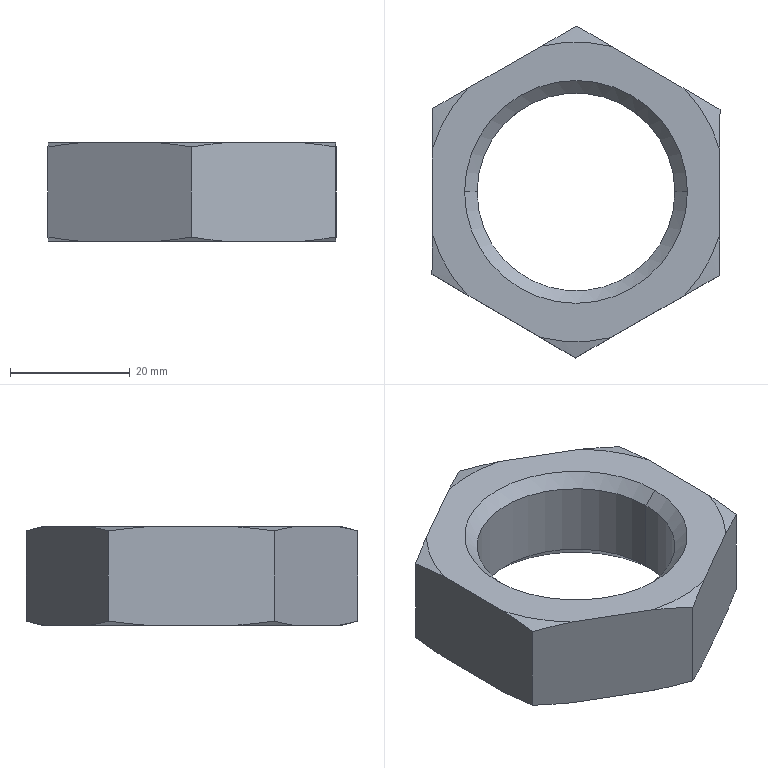Part | STEP file | GB/T 6173-M32×2_(M33) | 1 solid | 26 faces | box 48.06 x 55.37 x 16.5 mm | volume 18235 mm3 | cone 16 | plane 8 | cylinder 2 | commonest cylinder face diameters 33 x2
STEP:
#1=CARTESIAN_POINT('',(-16.5,0.,14.414));
#2=VERTEX_POINT('',#1);
#3=CARTESIAN_POINT('',(16.5,0.,14.414));
#4=VERTEX_POINT('',#3);
#5=CARTESIAN_POINT('',(0.,0.,14.414));
#6=DIRECTION('',(0.,0.,1.));
#7=DIRECTION('',(-1.,0.,0.));
#8=AXIS2_PLACEMENT_3D('',#5,#6,#7);
#9=CIRCLE('',#8,16.5);
#10=EDGE_CURVE('',#2,#4,#9,.T.);
#11=ORIENTED_EDGE('',*,*,#10,.F.);
#12=CARTESIAN_POINT('',(-18.586,0.,16.5));
#13=VERTEX_POINT('',#12);
#14=CARTESIAN_POINT('',(-16.5,0.,14.414));
#15=DIRECTION('',(-0.7071,0.,0.7071));
#16=VECTOR('',#15,1000.);
#17=LINE('',#14,#16);
#18=EDGE_CURVE('',#2,#13,#17,.T.);
#19=ORIENTED_EDGE('',*,*,#18,.T.);
#20=CARTESIAN_POINT('',(18.586,0.,16.5));
#21=VERTEX_POINT('',#20);
#22=CARTESIAN_POINT('',(0.,0.,16.5));
#23=DIRECTION('',(0.,0.,-1.));
#24=DIRECTION('',(-1.,0.,0.));
#25=AXIS2_PLACEMENT_3D('',#22,#23,#24);
#26=CIRCLE('',#25,18.586);
#27=EDGE_CURVE('',#21,#13,#26,.T.);
#28=ORIENTED_EDGE('',*,*,#27,.F.);
#29=CARTESIAN_POINT('',(16.5,0.,14.414));
#30=DIRECTION('',(0.7071,0.,0.7071));
#31=VECTOR('',#30,1000.);
#32=LINE('',#29,#31);
#33=EDGE_CURVE('',#4,#21,#32,.T.);
#34=ORIENTED_EDGE('',*,*,#33,.F.);
#35=EDGE_LOOP('',(#11,#19,#28,#34));
#36=FACE_OUTER_BOUND('',#35,.T.);
#37=CARTESIAN_POINT('',(0.,0.,14.414));
#38=DIRECTION('',(0.,0.,1.));
#39=DIRECTION('',(1.,0.,0.));
#40=AXIS2_PLACEMENT_3D('',#37,#38,#39);
#41=CONICAL_SURFACE('',#40,16.5,0.7854);
#42=ADVANCED_FACE('',(#36),#41,.F.);
#43=CARTESIAN_POINT('',(16.5,0.,2.086));
#44=VERTEX_POINT('',#43);
#45=CARTESIAN_POINT('',(-16.5,0.,2.086));
#46=VERTEX_POINT('',#45);
#47=CARTESIAN_POINT('',(0.,0.,2.086));
#48=DIRECTION('',(0.,0.,-1.));
#49=DIRECTION('',(-1.,0.,0.));
#50=AXIS2_PLACEMENT_3D('',#47,#48,#49);
#51=CIRCLE('',#50,16.5);
#52=EDGE_CURVE('',#44,#46,#51,.T.);
#53=ORIENTED_EDGE('',*,*,#52,.F.);
#54=CARTESIAN_POINT('',(18.586,0.,0.));
#55=VERTEX_POINT('',#54);
#56=CARTESIAN_POINT('',(18.586,0.,0.));
#57=DIRECTION('',(0.7071,0.,-0.7071));
#58=VECTOR('',#57,1000.);
#59=LINE('',#56,#58);
#60=EDGE_CURVE('',#44,#55,#59,.T.);
#61=ORIENTED_EDGE('',*,*,#60,.T.);
#62=CARTESIAN_POINT('',(-18.586,0.,0.));
#63=VERTEX_POINT('',#62);
#64=CARTESIAN_POINT('',(0.,0.,0.));
#65=DIRECTION('',(0.,0.,1.));
#66=DIRECTION('',(-1.,0.,0.));
#67=AXIS2_PLACEMENT_3D('',#64,#65,#66);
#68=CIRCLE('',#67,18.586);
#69=EDGE_CURVE('',#63,#55,#68,.T.);
#70=ORIENTED_EDGE('',*,*,#69,.F.);
#71=CARTESIAN_POINT('',(-18.586,0.,0.));
#72=DIRECTION('',(-0.7071,0.,-0.7071));
#73=VECTOR('',#72,1000.);
#74=LINE('',#71,#73);
#75=EDGE_CURVE('',#46,#63,#74,.T.);
#76=ORIENTED_EDGE('',*,*,#75,.F.);
#77=EDGE_LOOP('',(#53,#61,#70,#76));
#78=FACE_OUTER_BOUND('',#77,.T.);
#79=CARTESIAN_POINT('',(0.,0.,0.));
#80=DIRECTION('',(0.,0.,-1.));
#81=DIRECTION('',(-1.,0.,0.));
#82=AXIS2_PLACEMENT_3D('',#79,#80,#81);
#83=CONICAL_SURFACE('',#82,18.586,0.7854);
#84=ADVANCED_FACE('',(#78),#83,.F.);
#85=ORIENTED_EDGE('',*,*,#10,.T.);
#86=CARTESIAN_POINT('',(16.5,0.,16.5));
#87=DIRECTION('',(0.,0.,-1.));
#88=VECTOR('',#87,1000.);
#89=LINE('',#86,#88);
#90=EDGE_CURVE('',#4,#44,#89,.T.);
#91=ORIENTED_EDGE('',*,*,#90,.T.);
#92=ORIENTED_EDGE('',*,*,#52,.T.);
#93=CARTESIAN_POINT('',(-16.5,0.,16.5));
#94=DIRECTION('',(0.,0.,-1.));
#95=VECTOR('',#94,1000.);
#96=LINE('',#93,#95);
#97=EDGE_CURVE('',#2,#46,#96,.T.);
#98=ORIENTED_EDGE('',*,*,#97,.F.);
#99=EDGE_LOOP('',(#85,#91,#92,#98));
#100=FACE_OUTER_BOUND('',#99,.T.);
#101=CARTESIAN_POINT('',(0.,0.,16.5));
#102=DIRECTION('',(0.,0.,-1.));
#103=DIRECTION('',(-1.,0.,0.));
#104=AXIS2_PLACEMENT_3D('',#101,#102,#103);
#105=CYLINDRICAL_SURFACE('',#104,16.5);
#106=ADVANCED_FACE('',(#100),#105,.F.);
#107=CARTESIAN_POINT('',(24.03,13.748,15.781));
#108=VERTEX_POINT('',#107);
#109=CARTESIAN_POINT('',(18.189,17.151,16.5));
#110=VERTEX_POINT('',#109);
#111=CARTESIAN_POINT('',(24.03,13.748,15.781));
#112=CARTESIAN_POINT('',(22.089,14.879,16.082));
#113=CARTESIAN_POINT('',(20.142,16.013,16.328));
#114=CARTESIAN_POINT('',(18.189,17.151,16.5));
#115=B_SPLINE_CURVE_WITH_KNOTS('',3,(#111,#112,#113,#114),.UNSPECIFIED.,.F.,.F.,(4,4),(0.02271,0.02951),.UNSPECIFIED.);
#116=EDGE_CURVE('',#108,#110,#115,.T.);
#117=ORIENTED_EDGE('',*,*,#116,.F.);
#118=CARTESIAN_POINT('',(24.03,13.748,0.7194));
#119=VERTEX_POINT('',#118);
#120=CARTESIAN_POINT('',(24.03,13.748,16.5));
#121=DIRECTION('',(0.,0.,-1.));
#122=VECTOR('',#121,1000.);
#123=LINE('',#120,#122);
#124=EDGE_CURVE('',#108,#119,#123,.T.);
#125=ORIENTED_EDGE('',*,*,#124,.T.);
#126=CARTESIAN_POINT('',(18.189,17.151,0.));
#127=VERTEX_POINT('',#126);
#128=CARTESIAN_POINT('',(18.189,17.151,0.));
#129=CARTESIAN_POINT('',(19.165,16.582,0.08577));
#130=CARTESIAN_POINT('',(20.143,16.013,0.1906));
#131=CARTESIAN_POINT('',(22.09,14.879,0.4323));
#132=CARTESIAN_POINT('',(23.061,14.313,0.5692));
#133=CARTESIAN_POINT('',(24.03,13.748,0.7194));
#134=B_SPLINE_CURVE_WITH_KNOTS('',3,(#128,#129,#130,#131,#132,#133),.UNSPECIFIED.,.F.,.F.,(4,2,4),(0.04359,0.04693,0.05027),.UNSPECIFIED.);
#135=EDGE_CURVE('',#127,#119,#134,.T.);
#136=ORIENTED_EDGE('',*,*,#135,.F.);
#137=CARTESIAN_POINT('',(5.95,24.282,0.));
#138=VERTEX_POINT('',#137);
#139=CARTESIAN_POINT('',(24.03,13.748,0.));
#140=DIRECTION('',(-0.8641,0.5034,0.));
#141=VECTOR('',#140,1000.);
#142=LINE('',#139,#141);
#143=EDGE_CURVE('',#127,#138,#142,.T.);
#144=ORIENTED_EDGE('',*,*,#143,.T.);
#145=CARTESIAN_POINT('',(0.1089,27.685,0.7194));
#146=VERTEX_POINT('',#145);
#147=CARTESIAN_POINT('',(0.1089,27.685,0.7194));
#148=CARTESIAN_POINT('',(2.05,26.554,0.4184));
#149=CARTESIAN_POINT('',(3.997,25.42,0.1716));
#150=CARTESIAN_POINT('',(5.95,24.282,0.));
#151=B_SPLINE_CURVE_WITH_KNOTS('',3,(#147,#148,#149,#150),.UNSPECIFIED.,.F.,.F.,(4,4),(0.02271,0.02951),.UNSPECIFIED.);
#152=EDGE_CURVE('',#146,#138,#151,.T.);
#153=ORIENTED_EDGE('',*,*,#152,.F.);
#154=CARTESIAN_POINT('',(0.1089,27.685,15.781));
#155=VERTEX_POINT('',#154);
#156=CARTESIAN_POINT('',(0.1089,27.685,16.5));
#157=DIRECTION('',(0.,0.,-1.));
#158=VECTOR('',#157,1000.);
#159=LINE('',#156,#158);
#160=EDGE_CURVE('',#155,#146,#159,.T.);
#161=ORIENTED_EDGE('',*,*,#160,.F.);
#162=CARTESIAN_POINT('',(5.95,24.282,16.5));
#163=VERTEX_POINT('',#162);
#164=CARTESIAN_POINT('',(5.95,24.282,16.5));
#165=CARTESIAN_POINT('',(4.974,24.85,16.414));
#166=CARTESIAN_POINT('',(3.996,25.42,16.309));
#167=CARTESIAN_POINT('',(2.049,26.554,16.068));
#168=CARTESIAN_POINT('',(1.078,27.12,15.931));
#169=CARTESIAN_POINT('',(0.1089,27.685,15.781));
#170=B_SPLINE_CURVE_WITH_KNOTS('',3,(#164,#165,#166,#167,#168,#169),.UNSPECIFIED.,.F.,.F.,(4,2,4),(0.04359,0.04693,0.05027),.UNSPECIFIED.);
#171=EDGE_CURVE('',#163,#155,#170,.T.);
#172=ORIENTED_EDGE('',*,*,#171,.F.);
#173=CARTESIAN_POINT('',(24.03,13.748,16.5));
#174=DIRECTION('',(-0.8641,0.5034,0.));
#175=VECTOR('',#174,1000.);
#176=LINE('',#173,#175);
#177=EDGE_CURVE('',#110,#163,#176,.T.);
#178=ORIENTED_EDGE('',*,*,#177,.F.);
#179=EDGE_LOOP('',(#117,#125,#136,#144,#153,#161,#172,#178));
#180=FACE_OUTER_BOUND('',#179,.T.);
#181=CARTESIAN_POINT('',(24.03,13.748,16.5));
#182=DIRECTION('',(-0.5034,-0.8641,0.));
#183=DIRECTION('',(0.8641,-0.5034,0.));
#184=AXIS2_PLACEMENT_3D('',#181,#182,#183);
#185=PLANE('',#184);
#186=ADVANCED_FACE('',(#180),#185,.F.);
#187=CARTESIAN_POINT('',(-5.759,24.328,16.5));
#188=VERTEX_POINT('',#187);
#189=CARTESIAN_POINT('',(0.1089,27.685,15.781));
#190=CARTESIAN_POINT('',(-1.841,26.569,16.082));
#191=CARTESIAN_POINT('',(-3.797,25.45,16.328));
#192=CARTESIAN_POINT('',(-5.759,24.328,16.5));
#193=B_SPLINE_CURVE_WITH_KNOTS('',3,(#189,#190,#191,#192),.UNSPECIFIED.,.F.,.F.,(4,4),(0.0226,0.0294),.UNSPECIFIED.);
#194=EDGE_CURVE('',#155,#188,#193,.T.);
#195=ORIENTED_EDGE('',*,*,#194,.F.);
#196=ORIENTED_EDGE('',*,*,#160,.T.);
#197=CARTESIAN_POINT('',(-5.759,24.328,0.));
#198=VERTEX_POINT('',#197);
#199=CARTESIAN_POINT('',(-5.759,24.328,0.));
#200=CARTESIAN_POINT('',(-4.778,24.889,0.08577));
#201=CARTESIAN_POINT('',(-3.796,25.451,0.1906));
#202=CARTESIAN_POINT('',(-1.84,26.57,0.4323));
#203=CARTESIAN_POINT('',(-0.8647,27.128,0.5692));
#204=CARTESIAN_POINT('',(0.1089,27.685,0.7194));
#205=B_SPLINE_CURVE_WITH_KNOTS('',3,(#199,#200,#201,#202,#203,#204),.UNSPECIFIED.,.F.,.F.,(4,2,4),(0.04348,0.04682,0.05017),.UNSPECIFIED.);
#206=EDGE_CURVE('',#198,#146,#205,.T.);
#207=ORIENTED_EDGE('',*,*,#206,.F.);
#208=CARTESIAN_POINT('',(-18.053,17.294,0.));
#209=VERTEX_POINT('',#208);
#210=CARTESIAN_POINT('',(0.1089,27.685,0.));
#211=DIRECTION('',(-0.868,-0.4966,0.));
#212=VECTOR('',#211,1000.);
#213=LINE('',#210,#212);
#214=EDGE_CURVE('',#198,#209,#213,.T.);
#215=ORIENTED_EDGE('',*,*,#214,.T.);
#216=CARTESIAN_POINT('',(-23.921,13.937,0.7194));
#217=VERTEX_POINT('',#216);
#218=CARTESIAN_POINT('',(-23.921,13.937,0.7194));
#219=CARTESIAN_POINT('',(-21.971,15.052,0.4184));
#220=CARTESIAN_POINT('',(-20.016,16.171,0.1716));
#221=CARTESIAN_POINT('',(-18.053,17.294,0.));
#222=B_SPLINE_CURVE_WITH_KNOTS('',3,(#218,#219,#220,#221),.UNSPECIFIED.,.F.,.F.,(4,4),(0.0226,0.0294),.UNSPECIFIED.);
#223=EDGE_CURVE('',#217,#209,#222,.T.);
#224=ORIENTED_EDGE('',*,*,#223,.F.);
#225=CARTESIAN_POINT('',(-23.921,13.937,15.781));
#226=VERTEX_POINT('',#225);
#227=CARTESIAN_POINT('',(-23.921,13.937,16.5));
#228=DIRECTION('',(0.,0.,-1.));
#229=VECTOR('',#228,1000.);
#230=LINE('',#227,#229);
#231=EDGE_CURVE('',#226,#217,#230,.T.);
#232=ORIENTED_EDGE('',*,*,#231,.F.);
#233=CARTESIAN_POINT('',(-18.053,17.294,16.5));
#234=VERTEX_POINT('',#233);
#235=CARTESIAN_POINT('',(-18.053,17.294,16.5));
#236=CARTESIAN_POINT('',(-19.034,16.733,16.414));
#237=CARTESIAN_POINT('',(-20.016,16.171,16.309));
#238=CARTESIAN_POINT('',(-21.972,15.052,16.068));
#239=CARTESIAN_POINT('',(-22.948,14.494,15.931));
#240=CARTESIAN_POINT('',(-23.921,13.937,15.781));
#241=B_SPLINE_CURVE_WITH_KNOTS('',3,(#235,#236,#237,#238,#239,#240),.UNSPECIFIED.,.F.,.F.,(4,2,4),(0.04348,0.04682,0.05017),.UNSPECIFIED.);
#242=EDGE_CURVE('',#234,#226,#241,.T.);
#243=ORIENTED_EDGE('',*,*,#242,.F.);
#244=CARTESIAN_POINT('',(0.1089,27.685,16.5));
#245=DIRECTION('',(-0.868,-0.4966,0.));
#246=VECTOR('',#245,1000.);
#247=LINE('',#244,#246);
#248=EDGE_CURVE('',#188,#234,#247,.T.);
#249=ORIENTED_EDGE('',*,*,#248,.F.);
#250=EDGE_LOOP('',(#195,#196,#207,#215,#224,#232,#243,#249));
#251=FACE_OUTER_BOUND('',#250,.T.);
#252=CARTESIAN_POINT('',(0.1089,27.685,16.5));
#253=DIRECTION('',(0.4966,-0.868,0.));
#254=DIRECTION('',(0.868,0.4966,0.));
#255=AXIS2_PLACEMENT_3D('',#252,#253,#254);
#256=PLANE('',#255);
#257=ADVANCED_FACE('',(#251),#256,.F.);
#258=CARTESIAN_POINT('',(-23.948,7.176,16.5));
#259=VERTEX_POINT('',#258);
#260=CARTESIAN_POINT('',(-23.921,13.937,15.781));
#261=CARTESIAN_POINT('',(-23.93,11.689,16.082));
#262=CARTESIAN_POINT('',(-23.939,9.437,16.328));
#263=CARTESIAN_POINT('',(-23.948,7.176,16.5));
#264=B_SPLINE_CURVE_WITH_KNOTS('',3,(#260,#261,#262,#263),.UNSPECIFIED.,.F.,.F.,(4,4),(0.01959,0.02639),.UNSPECIFIED.);
#265=EDGE_CURVE('',#226,#259,#264,.T.);
#266=ORIENTED_EDGE('',*,*,#265,.F.);
#267=ORIENTED_EDGE('',*,*,#231,.T.);
#268=CARTESIAN_POINT('',(-23.948,7.176,0.));
#269=VERTEX_POINT('',#268);
#270=CARTESIAN_POINT('',(-23.948,7.176,0.));
#271=CARTESIAN_POINT('',(-23.943,8.305,0.08567));
#272=CARTESIAN_POINT('',(-23.939,9.436,0.1905));
#273=CARTESIAN_POINT('',(-23.93,11.69,0.4322));
#274=CARTESIAN_POINT('',(-23.926,12.815,0.5691));
#275=CARTESIAN_POINT('',(-23.921,13.937,0.7194));
#276=B_SPLINE_CURVE_WITH_KNOTS('',3,(#270,#271,#272,#273,#274,#275),.UNSPECIFIED.,.F.,.F.,(4,2,4),(0.04049,0.04383,0.04718),.UNSPECIFIED.);
#277=EDGE_CURVE('',#269,#217,#276,.T.);
#278=ORIENTED_EDGE('',*,*,#277,.F.);
#279=CARTESIAN_POINT('',(-24.004,-6.988,0.));
#280=VERTEX_POINT('',#279);
#281=CARTESIAN_POINT('',(-23.921,13.937,0.));
#282=DIRECTION('',(-0.003934,-1.,0.));
#283=VECTOR('',#282,1000.);
#284=LINE('',#281,#283);
#285=EDGE_CURVE('',#269,#280,#284,.T.);
#286=ORIENTED_EDGE('',*,*,#285,.T.);
#287=CARTESIAN_POINT('',(-24.03,-13.748,0.7194));
#288=VERTEX_POINT('',#287);
#289=CARTESIAN_POINT('',(-24.03,-13.748,0.7194));
#290=CARTESIAN_POINT('',(-24.021,-11.501,0.4184));
#291=CARTESIAN_POINT('',(-24.012,-9.248,0.1716));
#292=CARTESIAN_POINT('',(-24.004,-6.988,0.));
#293=B_SPLINE_CURVE_WITH_KNOTS('',3,(#289,#290,#291,#292),.UNSPECIFIED.,.F.,.F.,(4,4),(0.01959,0.02639),.UNSPECIFIED.);
#294=EDGE_CURVE('',#288,#280,#293,.T.);
#295=ORIENTED_EDGE('',*,*,#294,.F.);
#296=CARTESIAN_POINT('',(-24.03,-13.748,15.781));
#297=VERTEX_POINT('',#296);
#298=CARTESIAN_POINT('',(-24.03,-13.748,16.5));
#299=DIRECTION('',(0.,0.,-1.));
#300=VECTOR('',#299,1000.);
#301=LINE('',#298,#300);
#302=EDGE_CURVE('',#297,#288,#301,.T.);
#303=ORIENTED_EDGE('',*,*,#302,.F.);
#304=CARTESIAN_POINT('',(-24.004,-6.988,16.5));
#305=VERTEX_POINT('',#304);
#306=CARTESIAN_POINT('',(-24.004,-6.988,16.5));
#307=CARTESIAN_POINT('',(-24.008,-8.116,16.414));
#308=CARTESIAN_POINT('',(-24.012,-9.248,16.31));
#309=CARTESIAN_POINT('',(-24.021,-11.502,16.068));
#310=CARTESIAN_POINT('',(-24.026,-12.626,15.931));
#311=CARTESIAN_POINT('',(-24.03,-13.748,15.781));
#312=B_SPLINE_CURVE_WITH_KNOTS('',3,(#306,#307,#308,#309,#310,#311),.UNSPECIFIED.,.F.,.F.,(4,2,4),(0.04049,0.04383,0.04718),.UNSPECIFIED.);
#313=EDGE_CURVE('',#305,#297,#312,.T.);
#314=ORIENTED_EDGE('',*,*,#313,.F.);
#315=CARTESIAN_POINT('',(-23.921,13.937,16.5));
#316=DIRECTION('',(-0.003934,-1.,0.));
#317=VECTOR('',#316,1000.);
#318=LINE('',#315,#317);
#319=EDGE_CURVE('',#259,#305,#318,.T.);
#320=ORIENTED_EDGE('',*,*,#319,.F.);
#321=EDGE_LOOP('',(#266,#267,#278,#286,#295,#303,#314,#320));
#322=FACE_OUTER_BOUND('',#321,.T.);
#323=CARTESIAN_POINT('',(-23.921,13.937,16.5));
#324=DIRECTION('',(1.,-0.003934,0.));
#325=DIRECTION('',(0.003934,1.,0.));
#326=AXIS2_PLACEMENT_3D('',#323,#324,#325);
#327=PLANE('',#326);
#328=ADVANCED_FACE('',(#322),#327,.F.);
#329=CARTESIAN_POINT('',(-18.189,-17.151,16.5));
#330=VERTEX_POINT('',#329);
#331=CARTESIAN_POINT('',(-24.03,-13.748,15.781));
#332=CARTESIAN_POINT('',(-22.089,-14.879,16.082));
#333=CARTESIAN_POINT('',(-20.142,-16.013,16.328));
#334=CARTESIAN_POINT('',(-18.189,-17.151,16.5));
#335=B_SPLINE_CURVE_WITH_KNOTS('',3,(#331,#332,#333,#334),.UNSPECIFIED.,.F.,.F.,(4,4),(0.02271,0.02951),.UNSPECIFIED.);
#336=EDGE_CURVE('',#297,#330,#335,.T.);
#337=ORIENTED_EDGE('',*,*,#336,.F.);
#338=ORIENTED_EDGE('',*,*,#302,.T.);
#339=CARTESIAN_POINT('',(-18.189,-17.151,0.));
#340=VERTEX_POINT('',#339);
#341=CARTESIAN_POINT('',(-18.189,-17.151,0.));
#342=CARTESIAN_POINT('',(-19.165,-16.582,0.08577));
#343=CARTESIAN_POINT('',(-20.143,-16.013,0.1906));
#344=CARTESIAN_POINT('',(-22.09,-14.879,0.4323));
#345=CARTESIAN_POINT('',(-23.061,-14.313,0.5692));
#346=CARTESIAN_POINT('',(-24.03,-13.748,0.7194));
#347=B_SPLINE_CURVE_WITH_KNOTS('',3,(#341,#342,#343,#344,#345,#346),.UNSPECIFIED.,.F.,.F.,(4,2,4),(0.04359,0.04693,0.05027),.UNSPECIFIED.);
#348=EDGE_CURVE('',#340,#288,#347,.T.);
#349=ORIENTED_EDGE('',*,*,#348,.F.);
#350=CARTESIAN_POINT('',(-5.95,-24.282,0.));
#351=VERTEX_POINT('',#350);
#352=CARTESIAN_POINT('',(-24.03,-13.748,0.));
#353=DIRECTION('',(0.8641,-0.5034,0.));
#354=VECTOR('',#353,1000.);
#355=LINE('',#352,#354);
#356=EDGE_CURVE('',#340,#351,#355,.T.);
#357=ORIENTED_EDGE('',*,*,#356,.T.);
#358=CARTESIAN_POINT('',(-0.1089,-27.685,0.7194));
#359=VERTEX_POINT('',#358);
#360=CARTESIAN_POINT('',(-0.1089,-27.685,0.7194));
#361=CARTESIAN_POINT('',(-2.05,-26.554,0.4184));
#362=CARTESIAN_POINT('',(-3.997,-25.42,0.1716));
#363=CARTESIAN_POINT('',(-5.95,-24.282,0.));
#364=B_SPLINE_CURVE_WITH_KNOTS('',3,(#360,#361,#362,#363),.UNSPECIFIED.,.F.,.F.,(4,4),(0.02271,0.02951),.UNSPECIFIED.);
#365=EDGE_CURVE('',#359,#351,#364,.T.);
#366=ORIENTED_EDGE('',*,*,#365,.F.);
#367=CARTESIAN_POINT('',(-0.1089,-27.685,15.781));
#368=VERTEX_POINT('',#367);
#369=CARTESIAN_POINT('',(-0.1089,-27.685,16.5));
#370=DIRECTION('',(0.,0.,-1.));
#371=VECTOR('',#370,1000.);
#372=LINE('',#369,#371);
#373=EDGE_CURVE('',#368,#359,#372,.T.);
#374=ORIENTED_EDGE('',*,*,#373,.F.);
#375=CARTESIAN_POINT('',(-5.95,-24.282,16.5));
#376=VERTEX_POINT('',#375);
#377=CARTESIAN_POINT('',(-5.95,-24.282,16.5));
#378=CARTESIAN_POINT('',(-4.974,-24.85,16.414));
#379=CARTESIAN_POINT('',(-3.996,-25.42,16.309));
#380=CARTESIAN_POINT('',(-2.049,-26.554,16.068));
#381=CARTESIAN_POINT('',(-1.078,-27.12,15.931));
#382=CARTESIAN_POINT('',(-0.1089,-27.685,15.781));
#383=B_SPLINE_CURVE_WITH_KNOTS('',3,(#377,#378,#379,#380,#381,#382),.UNSPECIFIED.,.F.,.F.,(4,2,4),(0.04359,0.04693,0.05027),.UNSPECIFIED.);
#384=EDGE_CURVE('',#376,#368,#383,.T.);
#385=ORIENTED_EDGE('',*,*,#384,.F.);
#386=CARTESIAN_POINT('',(-24.03,-13.748,16.5));
#387=DIRECTION('',(0.8641,-0.5034,0.));
#388=VECTOR('',#387,1000.);
#389=LINE('',#386,#388);
#390=EDGE_CURVE('',#330,#376,#389,.T.);
#391=ORIENTED_EDGE('',*,*,#390,.F.);
#392=EDGE_LOOP('',(#337,#338,#349,#357,#366,#374,#385,#391));
#393=FACE_OUTER_BOUND('',#392,.T.);
#394=CARTESIAN_POINT('',(-24.03,-13.748,16.5));
#395=DIRECTION('',(0.5034,0.8641,0.));
#396=DIRECTION('',(-0.8641,0.5034,0.));
#397=AXIS2_PLACEMENT_3D('',#394,#395,#396);
#398=PLANE('',#397);
#399=ADVANCED_FACE('',(#393),#398,.F.);
#400=CARTESIAN_POINT('',(5.759,-24.328,16.5));
#401=VERTEX_POINT('',#400);
#402=CARTESIAN_POINT('',(-0.1089,-27.685,15.781));
#403=CARTESIAN_POINT('',(1.841,-26.569,16.082));
#404=CARTESIAN_POINT('',(3.797,-25.45,16.328));
#405=CARTESIAN_POINT('',(5.759,-24.328,16.5));
#406=B_SPLINE_CURVE_WITH_KNOTS('',3,(#402,#403,#404,#405),.UNSPECIFIED.,.F.,.F.,(4,4),(0.0226,0.0294),.UNSPECIFIED.);
#407=EDGE_CURVE('',#368,#401,#406,.T.);
#408=ORIENTED_EDGE('',*,*,#407,.F.);
#409=ORIENTED_EDGE('',*,*,#373,.T.);
#410=CARTESIAN_POINT('',(5.759,-24.328,0.));
#411=VERTEX_POINT('',#410);
#412=CARTESIAN_POINT('',(5.759,-24.328,0.));
#413=CARTESIAN_POINT('',(4.778,-24.889,0.08577));
#414=CARTESIAN_POINT('',(3.796,-25.451,0.1906));
#415=CARTESIAN_POINT('',(1.84,-26.57,0.4323));
#416=CARTESIAN_POINT('',(0.8647,-27.128,0.5692));
#417=CARTESIAN_POINT('',(-0.1089,-27.685,0.7194));
#418=B_SPLINE_CURVE_WITH_KNOTS('',3,(#412,#413,#414,#415,#416,#417),.UNSPECIFIED.,.F.,.F.,(4,2,4),(0.04348,0.04682,0.05017),.UNSPECIFIED.);
#419=EDGE_CURVE('',#411,#359,#418,.T.);
#420=ORIENTED_EDGE('',*,*,#419,.F.);
#421=CARTESIAN_POINT('',(18.053,-17.294,0.));
#422=VERTEX_POINT('',#421);
#423=CARTESIAN_POINT('',(-0.1089,-27.685,0.));
#424=DIRECTION('',(0.868,0.4966,0.));
#425=VECTOR('',#424,1000.);
#426=LINE('',#423,#425);
#427=EDGE_CURVE('',#411,#422,#426,.T.);
#428=ORIENTED_EDGE('',*,*,#427,.T.);
#429=CARTESIAN_POINT('',(23.921,-13.937,0.7194));
#430=VERTEX_POINT('',#429);
#431=CARTESIAN_POINT('',(23.921,-13.937,0.7194));
#432=CARTESIAN_POINT('',(21.971,-15.052,0.4184));
#433=CARTESIAN_POINT('',(20.016,-16.171,0.1716));
#434=CARTESIAN_POINT('',(18.053,-17.294,0.));
#435=B_SPLINE_CURVE_WITH_KNOTS('',3,(#431,#432,#433,#434),.UNSPECIFIED.,.F.,.F.,(4,4),(0.0226,0.0294),.UNSPECIFIED.);
#436=EDGE_CURVE('',#430,#422,#435,.T.);
#437=ORIENTED_EDGE('',*,*,#436,.F.);
#438=CARTESIAN_POINT('',(23.921,-13.937,15.781));
#439=VERTEX_POINT('',#438);
#440=CARTESIAN_POINT('',(23.921,-13.937,16.5));
#441=DIRECTION('',(0.,0.,-1.));
#442=VECTOR('',#441,1000.);
#443=LINE('',#440,#442);
#444=EDGE_CURVE('',#439,#430,#443,.T.);
#445=ORIENTED_EDGE('',*,*,#444,.F.);
#446=CARTESIAN_POINT('',(18.053,-17.294,16.5));
#447=VERTEX_POINT('',#446);
#448=CARTESIAN_POINT('',(18.053,-17.294,16.5));
#449=CARTESIAN_POINT('',(19.034,-16.733,16.414));
#450=CARTESIAN_POINT('',(20.016,-16.171,16.309));
#451=CARTESIAN_POINT('',(21.972,-15.052,16.068));
#452=CARTESIAN_POINT('',(22.948,-14.494,15.931));
#453=CARTESIAN_POINT('',(23.921,-13.937,15.781));
#454=B_SPLINE_CURVE_WITH_KNOTS('',3,(#448,#449,#450,#451,#452,#453),.UNSPECIFIED.,.F.,.F.,(4,2,4),(0.04348,0.04682,0.05017),.UNSPECIFIED.);
#455=EDGE_CURVE('',#447,#439,#454,.T.);
#456=ORIENTED_EDGE('',*,*,#455,.F.);
#457=CARTESIAN_POINT('',(-0.1089,-27.685,16.5));
#458=DIRECTION('',(0.868,0.4966,0.));
#459=VECTOR('',#458,1000.);
#460=LINE('',#457,#459);
#461=EDGE_CURVE('',#401,#447,#460,.T.);
#462=ORIENTED_EDGE('',*,*,#461,.F.);
#463=EDGE_LOOP('',(#408,#409,#420,#428,#437,#445,#456,#462));
#464=FACE_OUTER_BOUND('',#463,.T.);
#465=CARTESIAN_POINT('',(-0.1089,-27.685,16.5));
#466=DIRECTION('',(-0.4966,0.868,0.));
#467=DIRECTION('',(-0.868,-0.4966,0.));
#468=AXIS2_PLACEMENT_3D('',#465,#466,#467);
#469=PLANE('',#468);
#470=ADVANCED_FACE('',(#464),#469,.F.);
#471=CARTESIAN_POINT('',(23.948,-7.176,16.5));
#472=VERTEX_POINT('',#471);
#473=CARTESIAN_POINT('',(23.921,-13.937,15.781));
#474=CARTESIAN_POINT('',(23.93,-11.689,16.082));
#475=CARTESIAN_POINT('',(23.939,-9.437,16.328));
#476=CARTESIAN_POINT('',(23.948,-7.176,16.5));
#477=B_SPLINE_CURVE_WITH_KNOTS('',3,(#473,#474,#475,#476),.UNSPECIFIED.,.F.,.F.,(4,4),(0.01959,0.02639),.UNSPECIFIED.);
#478=EDGE_CURVE('',#439,#472,#477,.T.);
#479=ORIENTED_EDGE('',*,*,#478,.F.);
#480=ORIENTED_EDGE('',*,*,#444,.T.);
#481=CARTESIAN_POINT('',(23.948,-7.176,0.));
#482=VERTEX_POINT('',#481);
#483=CARTESIAN_POINT('',(23.948,-7.176,0.));
#484=CARTESIAN_POINT('',(23.943,-8.305,0.08567));
#485=CARTESIAN_POINT('',(23.939,-9.436,0.1905));
#486=CARTESIAN_POINT('',(23.93,-11.69,0.4322));
#487=CARTESIAN_POINT('',(23.926,-12.815,0.5691));
#488=CARTESIAN_POINT('',(23.921,-13.937,0.7194));
#489=B_SPLINE_CURVE_WITH_KNOTS('',3,(#483,#484,#485,#486,#487,#488),.UNSPECIFIED.,.F.,.F.,(4,2,4),(0.04049,0.04383,0.04718),.UNSPECIFIED.);
#490=EDGE_CURVE('',#482,#430,#489,.T.);
#491=ORIENTED_EDGE('',*,*,#490,.F.);
#492=CARTESIAN_POINT('',(24.004,6.988,0.));
#493=VERTEX_POINT('',#492);
#494=CARTESIAN_POINT('',(23.921,-13.937,0.));
#495=DIRECTION('',(0.003934,1.,0.));
#496=VECTOR('',#495,1000.);
#497=LINE('',#494,#496);
#498=EDGE_CURVE('',#482,#493,#497,.T.);
#499=ORIENTED_EDGE('',*,*,#498,.T.);
#500=CARTESIAN_POINT('',(24.03,13.748,0.7194));
#501=CARTESIAN_POINT('',(24.021,11.501,0.4184));
#502=CARTESIAN_POINT('',(24.012,9.248,0.1716));
#503=CARTESIAN_POINT('',(24.004,6.988,0.));
#504=B_SPLINE_CURVE_WITH_KNOTS('',3,(#500,#501,#502,#503),.UNSPECIFIED.,.F.,.F.,(4,4),(0.01959,0.02639),.UNSPECIFIED.);
#505=EDGE_CURVE('',#119,#493,#504,.T.);
#506=ORIENTED_EDGE('',*,*,#505,.F.);
#507=ORIENTED_EDGE('',*,*,#124,.F.);
#508=CARTESIAN_POINT('',(24.004,6.988,16.5));
#509=VERTEX_POINT('',#508);
#510=CARTESIAN_POINT('',(24.004,6.988,16.5));
#511=CARTESIAN_POINT('',(24.008,8.116,16.414));
#512=CARTESIAN_POINT('',(24.012,9.248,16.31));
#513=CARTESIAN_POINT('',(24.021,11.502,16.068));
#514=CARTESIAN_POINT('',(24.026,12.626,15.931));
#515=CARTESIAN_POINT('',(24.03,13.748,15.781));
#516=B_SPLINE_CURVE_WITH_KNOTS('',3,(#510,#511,#512,#513,#514,#515),.UNSPECIFIED.,.F.,.F.,(4,2,4),(0.04049,0.04383,0.04718),.UNSPECIFIED.);
#517=EDGE_CURVE('',#509,#108,#516,.T.);
#518=ORIENTED_EDGE('',*,*,#517,.F.);
#519=CARTESIAN_POINT('',(23.921,-13.937,16.5));
#520=DIRECTION('',(0.003934,1.,0.));
#521=VECTOR('',#520,1000.);
#522=LINE('',#519,#521);
#523=EDGE_CURVE('',#472,#509,#522,.T.);
#524=ORIENTED_EDGE('',*,*,#523,.F.);
#525=EDGE_LOOP('',(#479,#480,#491,#499,#506,#507,#518,#524));
#526=FACE_OUTER_BOUND('',#525,.T.);
#527=CARTESIAN_POINT('',(23.921,-13.937,16.5));
#528=DIRECTION('',(-1.,0.003934,0.));
#529=DIRECTION('',(-0.003934,-1.,0.));
#530=AXIS2_PLACEMENT_3D('',#527,#528,#529);
#531=PLANE('',#530);
#532=ADVANCED_FACE('',(#526),#531,.F.);
#533=ORIENTED_EDGE('',*,*,#27,.T.);
#534=CARTESIAN_POINT('',(0.,0.,16.5));
#535=DIRECTION('',(0.,0.,-1.));
#536=DIRECTION('',(-1.,0.,0.));
#537=AXIS2_PLACEMENT_3D('',#534,#535,#536);
#538=CIRCLE('',#537,18.586);
#539=EDGE_CURVE('',#13,#21,#538,.T.);
#540=ORIENTED_EDGE('',*,*,#539,.T.);
#541=EDGE_LOOP('',(#533,#540));
#542=FACE_BOUND('',#541,.T.);
#543=CARTESIAN_POINT('',(0.,0.,16.5));
#544=DIRECTION('',(0.,0.,-1.));
#545=DIRECTION('',(-1.,0.,0.));
#546=AXIS2_PLACEMENT_3D('',#543,#544,#545);
#547=CIRCLE('',#546,25.);
#548=EDGE_CURVE('',#259,#234,#547,.T.);
#549=ORIENTED_EDGE('',*,*,#548,.F.);
#550=ORIENTED_EDGE('',*,*,#319,.T.);
#551=CARTESIAN_POINT('',(0.,0.,16.5));
#552=DIRECTION('',(0.,0.,-1.));
#553=DIRECTION('',(-1.,0.,0.));
#554=AXIS2_PLACEMENT_3D('',#551,#552,#553);
#555=CIRCLE('',#554,25.);
#556=EDGE_CURVE('',#330,#305,#555,.T.);
#557=ORIENTED_EDGE('',*,*,#556,.F.);
#558=ORIENTED_EDGE('',*,*,#390,.T.);
#559=CARTESIAN_POINT('',(0.,0.,16.5));
#560=DIRECTION('',(0.,0.,-1.));
#561=DIRECTION('',(-1.,0.,0.));
#562=AXIS2_PLACEMENT_3D('',#559,#560,#561);
#563=CIRCLE('',#562,25.);
#564=EDGE_CURVE('',#401,#376,#563,.T.);
#565=ORIENTED_EDGE('',*,*,#564,.F.);
#566=ORIENTED_EDGE('',*,*,#461,.T.);
#567=CARTESIAN_POINT('',(0.,0.,16.5));
#568=DIRECTION('',(0.,0.,-1.));
#569=DIRECTION('',(-1.,0.,0.));
#570=AXIS2_PLACEMENT_3D('',#567,#568,#569);
#571=CIRCLE('',#570,25.);
#572=EDGE_CURVE('',#472,#447,#571,.T.);
#573=ORIENTED_EDGE('',*,*,#572,.F.);
#574=ORIENTED_EDGE('',*,*,#523,.T.);
#575=CARTESIAN_POINT('',(0.,0.,16.5));
#576=DIRECTION('',(0.,0.,1.));
#577=DIRECTION('',(1.,0.,0.));
#578=AXIS2_PLACEMENT_3D('',#575,#576,#577);
#579=CIRCLE('',#578,25.);
#580=EDGE_CURVE('',#509,#110,#579,.T.);
#581=ORIENTED_EDGE('',*,*,#580,.T.);
#582=ORIENTED_EDGE('',*,*,#177,.T.);
#583=CARTESIAN_POINT('',(0.,0.,16.5));
#584=DIRECTION('',(0.,0.,-1.));
#585=DIRECTION('',(-1.,0.,0.));
#586=AXIS2_PLACEMENT_3D('',#583,#584,#585);
#587=CIRCLE('',#586,25.);
#588=EDGE_CURVE('',#188,#163,#587,.T.);
#589=ORIENTED_EDGE('',*,*,#588,.F.);
#590=ORIENTED_EDGE('',*,*,#248,.T.);
#591=EDGE_LOOP('',(#549,#550,#557,#558,#565,#566,#573,#574,#581,#582,#589,#590));
#592=FACE_OUTER_BOUND('',#591,.T.);
#593=CARTESIAN_POINT('',(24.03,13.748,16.5));
#594=DIRECTION('',(0.,0.,-1.));
#595=DIRECTION('',(-1.,0.,0.));
#596=AXIS2_PLACEMENT_3D('',#593,#594,#595);
#597=PLANE('',#596);
#598=ADVANCED_FACE('',(#542,#592),#597,.F.);
#599=ORIENTED_EDGE('',*,*,#69,.T.);
#600=CARTESIAN_POINT('',(0.,0.,0.));
#601=DIRECTION('',(0.,0.,1.));
#602=DIRECTION('',(-1.,0.,0.));
#603=AXIS2_PLACEMENT_3D('',#600,#601,#602);
#604=CIRCLE('',#603,18.586);
#605=EDGE_CURVE('',#55,#63,#604,.T.);
#606=ORIENTED_EDGE('',*,*,#605,.T.);
#607=EDGE_LOOP('',(#599,#606));
#608=FACE_BOUND('',#607,.T.);
#609=ORIENTED_EDGE('',*,*,#285,.F.);
#610=CARTESIAN_POINT('',(0.,0.,0.));
#611=DIRECTION('',(0.,0.,-1.));
#612=DIRECTION('',(-1.,0.,0.));
#613=AXIS2_PLACEMENT_3D('',#610,#611,#612);
#614=CIRCLE('',#613,25.);
#615=EDGE_CURVE('',#269,#209,#614,.T.);
#616=ORIENTED_EDGE('',*,*,#615,.T.);
#617=ORIENTED_EDGE('',*,*,#214,.F.);
#618=CARTESIAN_POINT('',(0.,0.,0.));
#619=DIRECTION('',(0.,0.,-1.));
#620=DIRECTION('',(-1.,0.,0.));
#621=AXIS2_PLACEMENT_3D('',#618,#619,#620);
#622=CIRCLE('',#621,25.);
#623=EDGE_CURVE('',#198,#138,#622,.T.);
#624=ORIENTED_EDGE('',*,*,#623,.T.);
#625=ORIENTED_EDGE('',*,*,#143,.F.);
#626=CARTESIAN_POINT('',(0.,0.,0.));
#627=DIRECTION('',(0.,0.,-1.));
#628=DIRECTION('',(-1.,0.,0.));
#629=AXIS2_PLACEMENT_3D('',#626,#627,#628);
#630=CIRCLE('',#629,25.);
#631=EDGE_CURVE('',#127,#493,#630,.T.);
#632=ORIENTED_EDGE('',*,*,#631,.T.);
#633=ORIENTED_EDGE('',*,*,#498,.F.);
#634=CARTESIAN_POINT('',(0.,0.,0.));
#635=DIRECTION('',(0.,0.,-1.));
#636=DIRECTION('',(-1.,0.,0.));
#637=AXIS2_PLACEMENT_3D('',#634,#635,#636);
#638=CIRCLE('',#637,25.);
#639=EDGE_CURVE('',#482,#422,#638,.T.);
#640=ORIENTED_EDGE('',*,*,#639,.T.);
#641=ORIENTED_EDGE('',*,*,#427,.F.);
#642=CARTESIAN_POINT('',(0.,0.,0.));
#643=DIRECTION('',(0.,0.,-1.));
#644=DIRECTION('',(-1.,0.,0.));
#645=AXIS2_PLACEMENT_3D('',#642,#643,#644);
#646=CIRCLE('',#645,25.);
#647=EDGE_CURVE('',#411,#351,#646,.T.);
#648=ORIENTED_EDGE('',*,*,#647,.T.);
#649=ORIENTED_EDGE('',*,*,#356,.F.);
#650=CARTESIAN_POINT('',(0.,0.,0.));
#651=DIRECTION('',(0.,0.,-1.));
#652=DIRECTION('',(-1.,0.,0.));
#653=AXIS2_PLACEMENT_3D('',#650,#651,#652);
#654=CIRCLE('',#653,25.);
#655=EDGE_CURVE('',#340,#280,#654,.T.);
#656=ORIENTED_EDGE('',*,*,#655,.T.);
#657=EDGE_LOOP('',(#609,#616,#617,#624,#625,#632,#633,#640,#641,#648,#649,#656));
#658=FACE_OUTER_BOUND('',#657,.T.);
#659=CARTESIAN_POINT('',(24.03,13.748,0.));
#660=DIRECTION('',(0.,0.,-1.));
#661=DIRECTION('',(-1.,0.,0.));
#662=AXIS2_PLACEMENT_3D('',#659,#660,#661);
#663=PLANE('',#662);
#664=ADVANCED_FACE('',(#608,#658),#663,.T.);
#665=ORIENTED_EDGE('',*,*,#90,.F.);
#666=CARTESIAN_POINT('',(0.,0.,14.414));
#667=DIRECTION('',(0.,0.,1.));
#668=DIRECTION('',(-1.,0.,0.));
#669=AXIS2_PLACEMENT_3D('',#666,#667,#668);
#670=CIRCLE('',#669,16.5);
#671=EDGE_CURVE('',#4,#2,#670,.T.);
#672=ORIENTED_EDGE('',*,*,#671,.T.);
#673=ORIENTED_EDGE('',*,*,#97,.T.);
#674=CARTESIAN_POINT('',(0.,0.,2.086));
#675=DIRECTION('',(0.,0.,-1.));
#676=DIRECTION('',(-1.,0.,0.));
#677=AXIS2_PLACEMENT_3D('',#674,#675,#676);
#678=CIRCLE('',#677,16.5);
#679=EDGE_CURVE('',#46,#44,#678,.T.);
#680=ORIENTED_EDGE('',*,*,#679,.T.);
#681=EDGE_LOOP('',(#665,#672,#673,#680));
#682=FACE_OUTER_BOUND('',#681,.T.);
#683=CARTESIAN_POINT('',(0.,0.,16.5));
#684=DIRECTION('',(0.,0.,-1.));
#685=DIRECTION('',(-1.,0.,0.));
#686=AXIS2_PLACEMENT_3D('',#683,#684,#685);
#687=CYLINDRICAL_SURFACE('',#686,16.5);
#688=ADVANCED_FACE('',(#682),#687,.F.);
#689=ORIENTED_EDGE('',*,*,#436,.T.);
#690=ORIENTED_EDGE('',*,*,#639,.F.);
#691=ORIENTED_EDGE('',*,*,#490,.T.);
#692=EDGE_LOOP('',(#689,#690,#691));
#693=FACE_OUTER_BOUND('',#692,.T.);
#694=CARTESIAN_POINT('',(0.,0.,0.));
#695=DIRECTION('',(0.,0.,1.));
#696=DIRECTION('',(-1.,0.,0.));
#697=AXIS2_PLACEMENT_3D('',#694,#695,#696);
#698=CONICAL_SURFACE('',#697,25.,1.309);
#699=ADVANCED_FACE('',(#693),#698,.T.);
#700=ORIENTED_EDGE('',*,*,#135,.T.);
#701=ORIENTED_EDGE('',*,*,#505,.T.);
#702=ORIENTED_EDGE('',*,*,#631,.F.);
#703=EDGE_LOOP('',(#700,#701,#702));
#704=FACE_OUTER_BOUND('',#703,.T.);
#705=CARTESIAN_POINT('',(0.,0.,0.));
#706=DIRECTION('',(0.,0.,1.));
#707=DIRECTION('',(-1.,0.,0.));
#708=AXIS2_PLACEMENT_3D('',#705,#706,#707);
#709=CONICAL_SURFACE('',#708,25.,1.309);
#710=ADVANCED_FACE('',(#704),#709,.T.);
#711=ORIENTED_EDGE('',*,*,#365,.T.);
#712=ORIENTED_EDGE('',*,*,#647,.F.);
#713=ORIENTED_EDGE('',*,*,#419,.T.);
#714=EDGE_LOOP('',(#711,#712,#713));
#715=FACE_OUTER_BOUND('',#714,.T.);
#716=CARTESIAN_POINT('',(0.,0.,0.));
#717=DIRECTION('',(0.,0.,1.));
#718=DIRECTION('',(-1.,0.,0.));
#719=AXIS2_PLACEMENT_3D('',#716,#717,#718);
#720=CONICAL_SURFACE('',#719,25.,1.309);
#721=ADVANCED_FACE('',(#715),#720,.T.);
#722=ORIENTED_EDGE('',*,*,#294,.T.);
#723=ORIENTED_EDGE('',*,*,#655,.F.);
#724=ORIENTED_EDGE('',*,*,#348,.T.);
#725=EDGE_LOOP('',(#722,#723,#724));
#726=FACE_OUTER_BOUND('',#725,.T.);
#727=CARTESIAN_POINT('',(0.,0.,0.));
#728=DIRECTION('',(0.,0.,1.));
#729=DIRECTION('',(-1.,0.,0.));
#730=AXIS2_PLACEMENT_3D('',#727,#728,#729);
#731=CONICAL_SURFACE('',#730,25.,1.309);
#732=ADVANCED_FACE('',(#726),#731,.T.);
#733=ORIENTED_EDGE('',*,*,#223,.T.);
#734=ORIENTED_EDGE('',*,*,#615,.F.);
#735=ORIENTED_EDGE('',*,*,#277,.T.);
#736=EDGE_LOOP('',(#733,#734,#735));
#737=FACE_OUTER_BOUND('',#736,.T.);
#738=CARTESIAN_POINT('',(0.,0.,0.));
#739=DIRECTION('',(0.,0.,1.));
#740=DIRECTION('',(-1.,0.,0.));
#741=AXIS2_PLACEMENT_3D('',#738,#739,#740);
#742=CONICAL_SURFACE('',#741,25.,1.309);
#743=ADVANCED_FACE('',(#737),#742,.T.);
#744=ORIENTED_EDGE('',*,*,#152,.T.);
#745=ORIENTED_EDGE('',*,*,#623,.F.);
#746=ORIENTED_EDGE('',*,*,#206,.T.);
#747=EDGE_LOOP('',(#744,#745,#746));
#748=FACE_OUTER_BOUND('',#747,.T.);
#749=CARTESIAN_POINT('',(0.,0.,0.));
#750=DIRECTION('',(0.,0.,1.));
#751=DIRECTION('',(-1.,0.,0.));
#752=AXIS2_PLACEMENT_3D('',#749,#750,#751);
#753=CONICAL_SURFACE('',#752,25.,1.309);
#754=ADVANCED_FACE('',(#748),#753,.T.);
#755=ORIENTED_EDGE('',*,*,#313,.T.);
#756=ORIENTED_EDGE('',*,*,#336,.T.);
#757=ORIENTED_EDGE('',*,*,#556,.T.);
#758=EDGE_LOOP('',(#755,#756,#757));
#759=FACE_OUTER_BOUND('',#758,.T.);
#760=CARTESIAN_POINT('',(0.,0.,16.5));
#761=DIRECTION('',(0.,0.,-1.));
#762=DIRECTION('',(1.,0.,0.));
#763=AXIS2_PLACEMENT_3D('',#760,#761,#762);
#764=CONICAL_SURFACE('',#763,25.,1.309);
#765=ADVANCED_FACE('',(#759),#764,.T.);
#766=ORIENTED_EDGE('',*,*,#384,.T.);
#767=ORIENTED_EDGE('',*,*,#407,.T.);
#768=ORIENTED_EDGE('',*,*,#564,.T.);
#769=EDGE_LOOP('',(#766,#767,#768));
#770=FACE_OUTER_BOUND('',#769,.T.);
#771=CARTESIAN_POINT('',(0.,0.,16.5));
#772=DIRECTION('',(0.,0.,-1.));
#773=DIRECTION('',(1.,0.,0.));
#774=AXIS2_PLACEMENT_3D('',#771,#772,#773);
#775=CONICAL_SURFACE('',#774,25.,1.309);
#776=ADVANCED_FACE('',(#770),#775,.T.);
#777=ORIENTED_EDGE('',*,*,#455,.T.);
#778=ORIENTED_EDGE('',*,*,#478,.T.);
#779=ORIENTED_EDGE('',*,*,#572,.T.);
#780=EDGE_LOOP('',(#777,#778,#779));
#781=FACE_OUTER_BOUND('',#780,.T.);
#782=CARTESIAN_POINT('',(0.,0.,16.5));
#783=DIRECTION('',(0.,0.,-1.));
#784=DIRECTION('',(1.,0.,0.));
#785=AXIS2_PLACEMENT_3D('',#782,#783,#784);
#786=CONICAL_SURFACE('',#785,25.,1.309);
#787=ADVANCED_FACE('',(#781),#786,.T.);
#788=ORIENTED_EDGE('',*,*,#116,.T.);
#789=ORIENTED_EDGE('',*,*,#580,.F.);
#790=ORIENTED_EDGE('',*,*,#517,.T.);
#791=EDGE_LOOP('',(#788,#789,#790));
#792=FACE_OUTER_BOUND('',#791,.T.);
#793=CARTESIAN_POINT('',(0.,0.,16.5));
#794=DIRECTION('',(0.,0.,-1.));
#795=DIRECTION('',(1.,0.,0.));
#796=AXIS2_PLACEMENT_3D('',#793,#794,#795);
#797=CONICAL_SURFACE('',#796,25.,1.309);
#798=ADVANCED_FACE('',(#792),#797,.T.);
#799=ORIENTED_EDGE('',*,*,#171,.T.);
#800=ORIENTED_EDGE('',*,*,#194,.T.);
#801=ORIENTED_EDGE('',*,*,#588,.T.);
#802=EDGE_LOOP('',(#799,#800,#801));
#803=FACE_OUTER_BOUND('',#802,.T.);
#804=CARTESIAN_POINT('',(0.,0.,16.5));
#805=DIRECTION('',(0.,0.,-1.));
#806=DIRECTION('',(1.,0.,0.));
#807=AXIS2_PLACEMENT_3D('',#804,#805,#806);
#808=CONICAL_SURFACE('',#807,25.,1.309);
#809=ADVANCED_FACE('',(#803),#808,.T.);
#810=ORIENTED_EDGE('',*,*,#242,.T.);
#811=ORIENTED_EDGE('',*,*,#265,.T.);
#812=ORIENTED_EDGE('',*,*,#548,.T.);
#813=EDGE_LOOP('',(#810,#811,#812));
#814=FACE_OUTER_BOUND('',#813,.T.);
#815=CARTESIAN_POINT('',(0.,0.,16.5));
#816=DIRECTION('',(0.,0.,-1.));
#817=DIRECTION('',(1.,0.,0.));
#818=AXIS2_PLACEMENT_3D('',#815,#816,#817);
#819=CONICAL_SURFACE('',#818,25.,1.309);
#820=ADVANCED_FACE('',(#814),#819,.T.);
#821=ORIENTED_EDGE('',*,*,#60,.F.);
#822=ORIENTED_EDGE('',*,*,#679,.F.);
#823=ORIENTED_EDGE('',*,*,#75,.T.);
#824=ORIENTED_EDGE('',*,*,#605,.F.);
#825=EDGE_LOOP('',(#821,#822,#823,#824));
#826=FACE_OUTER_BOUND('',#825,.T.);
#827=CARTESIAN_POINT('',(0.,0.,0.));
#828=DIRECTION('',(0.,0.,-1.));
#829=DIRECTION('',(-1.,0.,0.));
#830=AXIS2_PLACEMENT_3D('',#827,#828,#829);
#831=CONICAL_SURFACE('',#830,18.586,0.7854);
#832=ADVANCED_FACE('',(#826),#831,.F.);
#833=ORIENTED_EDGE('',*,*,#18,.F.);
#834=ORIENTED_EDGE('',*,*,#671,.F.);
#835=ORIENTED_EDGE('',*,*,#33,.T.);
#836=ORIENTED_EDGE('',*,*,#539,.F.);
#837=EDGE_LOOP('',(#833,#834,#835,#836));
#838=FACE_OUTER_BOUND('',#837,.T.);
#839=CARTESIAN_POINT('',(0.,0.,14.414));
#840=DIRECTION('',(0.,0.,1.));
#841=DIRECTION('',(1.,0.,0.));
#842=AXIS2_PLACEMENT_3D('',#839,#840,#841);
#843=CONICAL_SURFACE('',#842,16.5,0.7854);
#844=ADVANCED_FACE('',(#838),#843,.F.);
#845=CLOSED_SHELL('',(#42,#84,#106,#186,#257,#328,#399,#470,#532,#598,#664,#688,#699,#710,#721,#732,#743,#754,#765,#776,#787,#798,#809,#820,#832,#844));
#846=MANIFOLD_SOLID_BREP('',#845);
#847=CARTESIAN_POINT('',(0.,0.,0.));
#848=DIRECTION('',(0.,0.,1.));
#849=DIRECTION('',(1.,0.,0.));
#850=AXIS2_PLACEMENT_3D('',#847,#848,#849);
#851=(LENGTH_UNIT()NAMED_UNIT(*)SI_UNIT(.MILLI.,.METRE.));
#852=UNCERTAINTY_MEASURE_WITH_UNIT(LENGTH_MEASURE(0.00001),#851,'','');
#853=(NAMED_UNIT(*)PLANE_ANGLE_UNIT()SI_UNIT($,.RADIAN.));
#854=(NAMED_UNIT(*)SI_UNIT($,.STERADIAN.)SOLID_ANGLE_UNIT());
#855=(GEOMETRIC_REPRESENTATION_CONTEXT(3)GLOBAL_UNCERTAINTY_ASSIGNED_CONTEXT((#852))GLOBAL_UNIT_ASSIGNED_CONTEXT((#851,#853,#854))REPRESENTATION_CONTEXT('',''));
#856=ADVANCED_BREP_SHAPE_REPRESENTATION('',(#846,#850),#855);